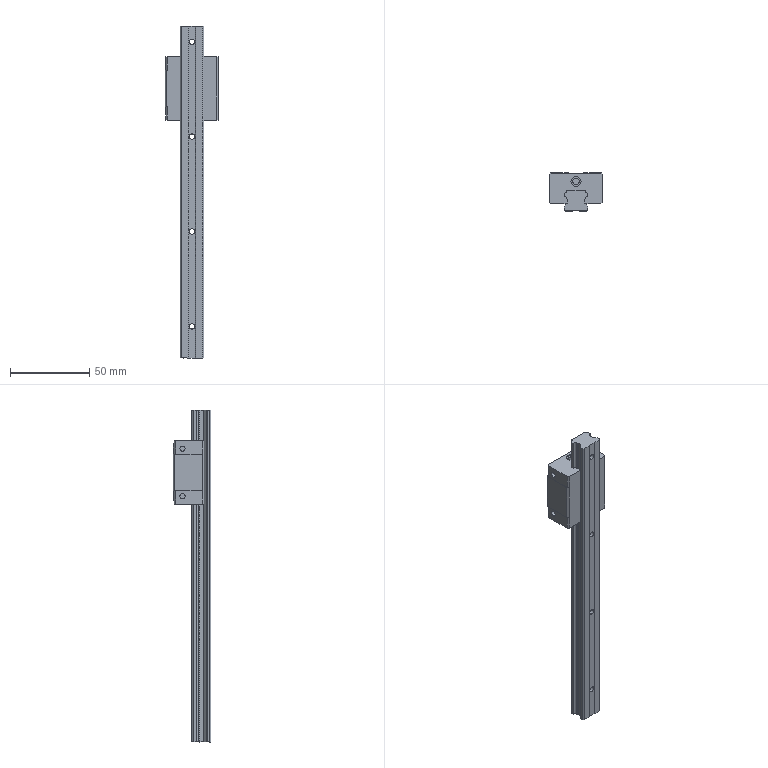Part | SolidWorks | 2 solids | 176 faces | box 34 x 24 x 210 mm | volume 54732 mm3 | plane 91 | cylinder 85 | commonest cylinder face diameters 6.5 x12 0.6 x11 3 x10 0.46 x8 3.35 x8 4 x8